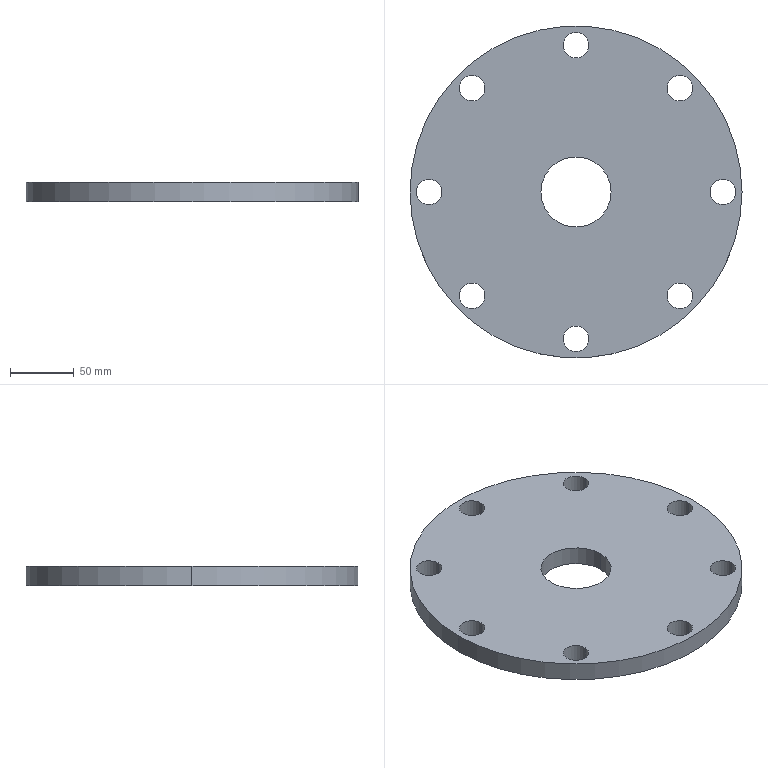Part | SolidWorks | features CirPattern 1, Cut 1, Extrusion 1 | 1 solid | 22 faces | box 260 x 260 x 15 mm | volume 723057 mm3 | cylinder 20 | plane 2 | commonest cylinder face diameters 20 x16 55 x2 260 x2
STEP:
#1=CARTESIAN_POINT('',(-10.,115.,0.));
#2=VERTEX_POINT('',#1);
#3=CARTESIAN_POINT('',(10.,115.,0.));
#4=VERTEX_POINT('',#3);
#5=CARTESIAN_POINT('',(0.,115.,0.));
#6=DIRECTION('',(0.,0.,1.));
#7=DIRECTION('',(1.,0.,0.));
#8=AXIS2_PLACEMENT_3D('',#5,#6,#7);
#9=CIRCLE('',#8,10.);
#10=EDGE_CURVE('',#2,#4,#9,.T.);
#11=ORIENTED_EDGE('',*,*,#10,.F.);
#12=CARTESIAN_POINT('',(-10.,115.,15.));
#13=VERTEX_POINT('',#12);
#14=CARTESIAN_POINT('',(-10.,115.,-0.000012));
#15=DIRECTION('',(0.,0.,1.));
#16=VECTOR('',#15,1000.);
#17=LINE('',#14,#16);
#18=EDGE_CURVE('',#2,#13,#17,.T.);
#19=ORIENTED_EDGE('',*,*,#18,.T.);
#20=CARTESIAN_POINT('',(10.,115.,15.));
#21=VERTEX_POINT('',#20);
#22=CARTESIAN_POINT('',(0.,115.,15.));
#23=DIRECTION('',(0.,0.,1.));
#24=DIRECTION('',(0.,-1.,0.));
#25=AXIS2_PLACEMENT_3D('',#22,#23,#24);
#26=CIRCLE('',#25,10.);
#27=EDGE_CURVE('',#13,#21,#26,.T.);
#28=ORIENTED_EDGE('',*,*,#27,.T.);
#29=CARTESIAN_POINT('',(10.,115.,-0.000012));
#30=DIRECTION('',(0.,0.,1.));
#31=VECTOR('',#30,1000.);
#32=LINE('',#29,#31);
#33=EDGE_CURVE('',#4,#21,#32,.T.);
#34=ORIENTED_EDGE('',*,*,#33,.F.);
#35=EDGE_LOOP('',(#11,#19,#28,#34));
#36=FACE_OUTER_BOUND('',#35,.T.);
#37=CARTESIAN_POINT('',(0.,115.,-0.000012));
#38=DIRECTION('',(0.,0.,1.));
#39=DIRECTION('',(1.,0.,0.));
#40=AXIS2_PLACEMENT_3D('',#37,#38,#39);
#41=CYLINDRICAL_SURFACE('',#40,10.);
#42=ADVANCED_FACE('',(#36),#41,.F.);
#43=CARTESIAN_POINT('',(71.317,81.317,0.));
#44=VERTEX_POINT('',#43);
#45=CARTESIAN_POINT('',(91.317,81.317,0.));
#46=VERTEX_POINT('',#45);
#47=CARTESIAN_POINT('',(81.317,81.317,0.));
#48=DIRECTION('',(0.,0.,1.));
#49=DIRECTION('',(1.,0.,0.));
#50=AXIS2_PLACEMENT_3D('',#47,#48,#49);
#51=CIRCLE('',#50,10.);
#52=EDGE_CURVE('',#44,#46,#51,.T.);
#53=ORIENTED_EDGE('',*,*,#52,.F.);
#54=CARTESIAN_POINT('',(71.317,81.317,15.));
#55=VERTEX_POINT('',#54);
#56=CARTESIAN_POINT('',(71.317,81.317,-0.000012));
#57=DIRECTION('',(0.,0.,1.));
#58=VECTOR('',#57,1000.);
#59=LINE('',#56,#58);
#60=EDGE_CURVE('',#44,#55,#59,.T.);
#61=ORIENTED_EDGE('',*,*,#60,.T.);
#62=CARTESIAN_POINT('',(91.317,81.317,15.));
#63=VERTEX_POINT('',#62);
#64=CARTESIAN_POINT('',(81.317,81.317,15.));
#65=DIRECTION('',(0.,0.,1.));
#66=DIRECTION('',(-0.7071,-0.7071,0.));
#67=AXIS2_PLACEMENT_3D('',#64,#65,#66);
#68=CIRCLE('',#67,10.);
#69=EDGE_CURVE('',#55,#63,#68,.T.);
#70=ORIENTED_EDGE('',*,*,#69,.T.);
#71=CARTESIAN_POINT('',(91.317,81.317,-0.000012));
#72=DIRECTION('',(0.,0.,1.));
#73=VECTOR('',#72,1000.);
#74=LINE('',#71,#73);
#75=EDGE_CURVE('',#46,#63,#74,.T.);
#76=ORIENTED_EDGE('',*,*,#75,.F.);
#77=EDGE_LOOP('',(#53,#61,#70,#76));
#78=FACE_OUTER_BOUND('',#77,.T.);
#79=CARTESIAN_POINT('',(81.317,81.317,-0.000012));
#80=DIRECTION('',(0.,0.,1.));
#81=DIRECTION('',(1.,0.,0.));
#82=AXIS2_PLACEMENT_3D('',#79,#80,#81);
#83=CYLINDRICAL_SURFACE('',#82,10.);
#84=ADVANCED_FACE('',(#78),#83,.F.);
#85=CARTESIAN_POINT('',(105.,0.,0.));
#86=VERTEX_POINT('',#85);
#87=CARTESIAN_POINT('',(125.,0.,0.));
#88=VERTEX_POINT('',#87);
#89=CARTESIAN_POINT('',(115.,0.,0.));
#90=DIRECTION('',(0.,0.,1.));
#91=DIRECTION('',(1.,0.,0.));
#92=AXIS2_PLACEMENT_3D('',#89,#90,#91);
#93=CIRCLE('',#92,10.);
#94=EDGE_CURVE('',#86,#88,#93,.T.);
#95=ORIENTED_EDGE('',*,*,#94,.F.);
#96=CARTESIAN_POINT('',(105.,0.,15.));
#97=VERTEX_POINT('',#96);
#98=CARTESIAN_POINT('',(105.,0.,-0.000012));
#99=DIRECTION('',(0.,0.,1.));
#100=VECTOR('',#99,1000.);
#101=LINE('',#98,#100);
#102=EDGE_CURVE('',#86,#97,#101,.T.);
#103=ORIENTED_EDGE('',*,*,#102,.T.);
#104=CARTESIAN_POINT('',(125.,0.,15.));
#105=VERTEX_POINT('',#104);
#106=CARTESIAN_POINT('',(115.,0.,15.));
#107=DIRECTION('',(0.,0.,1.));
#108=DIRECTION('',(-1.,0.,0.));
#109=AXIS2_PLACEMENT_3D('',#106,#107,#108);
#110=CIRCLE('',#109,10.);
#111=EDGE_CURVE('',#97,#105,#110,.T.);
#112=ORIENTED_EDGE('',*,*,#111,.T.);
#113=CARTESIAN_POINT('',(125.,0.,-0.000012));
#114=DIRECTION('',(0.,0.,1.));
#115=VECTOR('',#114,1000.);
#116=LINE('',#113,#115);
#117=EDGE_CURVE('',#88,#105,#116,.T.);
#118=ORIENTED_EDGE('',*,*,#117,.F.);
#119=EDGE_LOOP('',(#95,#103,#112,#118));
#120=FACE_OUTER_BOUND('',#119,.T.);
#121=CARTESIAN_POINT('',(115.,0.,-0.000012));
#122=DIRECTION('',(0.,0.,1.));
#123=DIRECTION('',(1.,0.,0.));
#124=AXIS2_PLACEMENT_3D('',#121,#122,#123);
#125=CYLINDRICAL_SURFACE('',#124,10.);
#126=ADVANCED_FACE('',(#120),#125,.F.);
#127=CARTESIAN_POINT('',(71.317,-81.317,0.));
#128=VERTEX_POINT('',#127);
#129=CARTESIAN_POINT('',(91.317,-81.317,0.));
#130=VERTEX_POINT('',#129);
#131=CARTESIAN_POINT('',(81.317,-81.317,0.));
#132=DIRECTION('',(0.,0.,1.));
#133=DIRECTION('',(1.,0.,0.));
#134=AXIS2_PLACEMENT_3D('',#131,#132,#133);
#135=CIRCLE('',#134,10.);
#136=EDGE_CURVE('',#128,#130,#135,.T.);
#137=ORIENTED_EDGE('',*,*,#136,.F.);
#138=CARTESIAN_POINT('',(71.317,-81.317,15.));
#139=VERTEX_POINT('',#138);
#140=CARTESIAN_POINT('',(71.317,-81.317,-0.000012));
#141=DIRECTION('',(0.,0.,1.));
#142=VECTOR('',#141,1000.);
#143=LINE('',#140,#142);
#144=EDGE_CURVE('',#128,#139,#143,.T.);
#145=ORIENTED_EDGE('',*,*,#144,.T.);
#146=CARTESIAN_POINT('',(91.317,-81.317,15.));
#147=VERTEX_POINT('',#146);
#148=CARTESIAN_POINT('',(81.317,-81.317,15.));
#149=DIRECTION('',(0.,0.,1.));
#150=DIRECTION('',(-0.7071,0.7071,0.));
#151=AXIS2_PLACEMENT_3D('',#148,#149,#150);
#152=CIRCLE('',#151,10.);
#153=EDGE_CURVE('',#139,#147,#152,.T.);
#154=ORIENTED_EDGE('',*,*,#153,.T.);
#155=CARTESIAN_POINT('',(91.317,-81.317,-0.000012));
#156=DIRECTION('',(0.,0.,1.));
#157=VECTOR('',#156,1000.);
#158=LINE('',#155,#157);
#159=EDGE_CURVE('',#130,#147,#158,.T.);
#160=ORIENTED_EDGE('',*,*,#159,.F.);
#161=EDGE_LOOP('',(#137,#145,#154,#160));
#162=FACE_OUTER_BOUND('',#161,.T.);
#163=CARTESIAN_POINT('',(81.317,-81.317,-0.000012));
#164=DIRECTION('',(0.,0.,1.));
#165=DIRECTION('',(1.,0.,0.));
#166=AXIS2_PLACEMENT_3D('',#163,#164,#165);
#167=CYLINDRICAL_SURFACE('',#166,10.);
#168=ADVANCED_FACE('',(#162),#167,.F.);
#169=CARTESIAN_POINT('',(-10.,-115.,0.));
#170=VERTEX_POINT('',#169);
#171=CARTESIAN_POINT('',(10.,-115.,0.));
#172=VERTEX_POINT('',#171);
#173=CARTESIAN_POINT('',(0.,-115.,0.));
#174=DIRECTION('',(0.,0.,1.));
#175=DIRECTION('',(1.,0.,0.));
#176=AXIS2_PLACEMENT_3D('',#173,#174,#175);
#177=CIRCLE('',#176,10.);
#178=EDGE_CURVE('',#170,#172,#177,.T.);
#179=ORIENTED_EDGE('',*,*,#178,.F.);
#180=CARTESIAN_POINT('',(-10.,-115.,15.));
#181=VERTEX_POINT('',#180);
#182=CARTESIAN_POINT('',(-10.,-115.,-0.000012));
#183=DIRECTION('',(0.,0.,1.));
#184=VECTOR('',#183,1000.);
#185=LINE('',#182,#184);
#186=EDGE_CURVE('',#170,#181,#185,.T.);
#187=ORIENTED_EDGE('',*,*,#186,.T.);
#188=CARTESIAN_POINT('',(10.,-115.,15.));
#189=VERTEX_POINT('',#188);
#190=CARTESIAN_POINT('',(0.,-115.,15.));
#191=DIRECTION('',(0.,0.,1.));
#192=DIRECTION('',(0.,1.,0.));
#193=AXIS2_PLACEMENT_3D('',#190,#191,#192);
#194=CIRCLE('',#193,10.);
#195=EDGE_CURVE('',#181,#189,#194,.T.);
#196=ORIENTED_EDGE('',*,*,#195,.T.);
#197=CARTESIAN_POINT('',(10.,-115.,-0.000012));
#198=DIRECTION('',(0.,0.,1.));
#199=VECTOR('',#198,1000.);
#200=LINE('',#197,#199);
#201=EDGE_CURVE('',#172,#189,#200,.T.);
#202=ORIENTED_EDGE('',*,*,#201,.F.);
#203=EDGE_LOOP('',(#179,#187,#196,#202));
#204=FACE_OUTER_BOUND('',#203,.T.);
#205=CARTESIAN_POINT('',(0.,-115.,-0.000012));
#206=DIRECTION('',(0.,0.,1.));
#207=DIRECTION('',(1.,0.,0.));
#208=AXIS2_PLACEMENT_3D('',#205,#206,#207);
#209=CYLINDRICAL_SURFACE('',#208,10.);
#210=ADVANCED_FACE('',(#204),#209,.F.);
#211=CARTESIAN_POINT('',(-91.317,-81.317,0.));
#212=VERTEX_POINT('',#211);
#213=CARTESIAN_POINT('',(-71.317,-81.317,0.));
#214=VERTEX_POINT('',#213);
#215=CARTESIAN_POINT('',(-81.317,-81.317,0.));
#216=DIRECTION('',(0.,0.,1.));
#217=DIRECTION('',(1.,0.,0.));
#218=AXIS2_PLACEMENT_3D('',#215,#216,#217);
#219=CIRCLE('',#218,10.);
#220=EDGE_CURVE('',#212,#214,#219,.T.);
#221=ORIENTED_EDGE('',*,*,#220,.F.);
#222=CARTESIAN_POINT('',(-91.317,-81.317,15.));
#223=VERTEX_POINT('',#222);
#224=CARTESIAN_POINT('',(-91.317,-81.317,-0.000012));
#225=DIRECTION('',(0.,0.,1.));
#226=VECTOR('',#225,1000.);
#227=LINE('',#224,#226);
#228=EDGE_CURVE('',#212,#223,#227,.T.);
#229=ORIENTED_EDGE('',*,*,#228,.T.);
#230=CARTESIAN_POINT('',(-71.317,-81.317,15.));
#231=VERTEX_POINT('',#230);
#232=CARTESIAN_POINT('',(-81.317,-81.317,15.));
#233=DIRECTION('',(0.,0.,1.));
#234=DIRECTION('',(0.7071,0.7071,0.));
#235=AXIS2_PLACEMENT_3D('',#232,#233,#234);
#236=CIRCLE('',#235,10.);
#237=EDGE_CURVE('',#223,#231,#236,.T.);
#238=ORIENTED_EDGE('',*,*,#237,.T.);
#239=CARTESIAN_POINT('',(-71.317,-81.317,-0.000012));
#240=DIRECTION('',(0.,0.,1.));
#241=VECTOR('',#240,1000.);
#242=LINE('',#239,#241);
#243=EDGE_CURVE('',#214,#231,#242,.T.);
#244=ORIENTED_EDGE('',*,*,#243,.F.);
#245=EDGE_LOOP('',(#221,#229,#238,#244));
#246=FACE_OUTER_BOUND('',#245,.T.);
#247=CARTESIAN_POINT('',(-81.317,-81.317,-0.000012));
#248=DIRECTION('',(0.,0.,1.));
#249=DIRECTION('',(1.,0.,0.));
#250=AXIS2_PLACEMENT_3D('',#247,#248,#249);
#251=CYLINDRICAL_SURFACE('',#250,10.);
#252=ADVANCED_FACE('',(#246),#251,.F.);
#253=CARTESIAN_POINT('',(-91.317,81.317,0.));
#254=VERTEX_POINT('',#253);
#255=CARTESIAN_POINT('',(-71.317,81.317,0.));
#256=VERTEX_POINT('',#255);
#257=CARTESIAN_POINT('',(-81.317,81.317,0.));
#258=DIRECTION('',(0.,0.,1.));
#259=DIRECTION('',(1.,0.,0.));
#260=AXIS2_PLACEMENT_3D('',#257,#258,#259);
#261=CIRCLE('',#260,10.);
#262=EDGE_CURVE('',#254,#256,#261,.T.);
#263=ORIENTED_EDGE('',*,*,#262,.F.);
#264=CARTESIAN_POINT('',(-91.317,81.317,15.));
#265=VERTEX_POINT('',#264);
#266=CARTESIAN_POINT('',(-91.317,81.317,-0.000012));
#267=DIRECTION('',(0.,0.,1.));
#268=VECTOR('',#267,1000.);
#269=LINE('',#266,#268);
#270=EDGE_CURVE('',#254,#265,#269,.T.);
#271=ORIENTED_EDGE('',*,*,#270,.T.);
#272=CARTESIAN_POINT('',(-71.317,81.317,15.));
#273=VERTEX_POINT('',#272);
#274=CARTESIAN_POINT('',(-81.317,81.317,15.));
#275=DIRECTION('',(0.,0.,1.));
#276=DIRECTION('',(0.7071,-0.7071,0.));
#277=AXIS2_PLACEMENT_3D('',#274,#275,#276);
#278=CIRCLE('',#277,10.);
#279=EDGE_CURVE('',#265,#273,#278,.T.);
#280=ORIENTED_EDGE('',*,*,#279,.T.);
#281=CARTESIAN_POINT('',(-71.317,81.317,-0.000012));
#282=DIRECTION('',(0.,0.,1.));
#283=VECTOR('',#282,1000.);
#284=LINE('',#281,#283);
#285=EDGE_CURVE('',#256,#273,#284,.T.);
#286=ORIENTED_EDGE('',*,*,#285,.F.);
#287=EDGE_LOOP('',(#263,#271,#280,#286));
#288=FACE_OUTER_BOUND('',#287,.T.);
#289=CARTESIAN_POINT('',(-81.317,81.317,-0.000012));
#290=DIRECTION('',(0.,0.,1.));
#291=DIRECTION('',(1.,0.,0.));
#292=AXIS2_PLACEMENT_3D('',#289,#290,#291);
#293=CYLINDRICAL_SURFACE('',#292,10.);
#294=ADVANCED_FACE('',(#288),#293,.F.);
#295=CARTESIAN_POINT('',(-125.,0.,0.));
#296=VERTEX_POINT('',#295);
#297=CARTESIAN_POINT('',(-105.,0.,0.));
#298=VERTEX_POINT('',#297);
#299=CARTESIAN_POINT('',(-115.,0.,0.));
#300=DIRECTION('',(0.,0.,1.));
#301=DIRECTION('',(1.,0.,0.));
#302=AXIS2_PLACEMENT_3D('',#299,#300,#301);
#303=CIRCLE('',#302,10.);
#304=EDGE_CURVE('',#296,#298,#303,.T.);
#305=ORIENTED_EDGE('',*,*,#304,.F.);
#306=CARTESIAN_POINT('',(-125.,0.,15.));
#307=VERTEX_POINT('',#306);
#308=CARTESIAN_POINT('',(-125.,0.,-0.000012));
#309=DIRECTION('',(0.,0.,1.));
#310=VECTOR('',#309,1000.);
#311=LINE('',#308,#310);
#312=EDGE_CURVE('',#296,#307,#311,.T.);
#313=ORIENTED_EDGE('',*,*,#312,.T.);
#314=CARTESIAN_POINT('',(-105.,0.,15.));
#315=VERTEX_POINT('',#314);
#316=CARTESIAN_POINT('',(-115.,0.,15.));
#317=DIRECTION('',(0.,0.,1.));
#318=DIRECTION('',(1.,0.,0.));
#319=AXIS2_PLACEMENT_3D('',#316,#317,#318);
#320=CIRCLE('',#319,10.);
#321=EDGE_CURVE('',#307,#315,#320,.T.);
#322=ORIENTED_EDGE('',*,*,#321,.T.);
#323=CARTESIAN_POINT('',(-105.,0.,-0.000012));
#324=DIRECTION('',(0.,0.,1.));
#325=VECTOR('',#324,1000.);
#326=LINE('',#323,#325);
#327=EDGE_CURVE('',#298,#315,#326,.T.);
#328=ORIENTED_EDGE('',*,*,#327,.F.);
#329=EDGE_LOOP('',(#305,#313,#322,#328));
#330=FACE_OUTER_BOUND('',#329,.T.);
#331=CARTESIAN_POINT('',(-115.,0.,-0.000012));
#332=DIRECTION('',(0.,0.,1.));
#333=DIRECTION('',(1.,0.,0.));
#334=AXIS2_PLACEMENT_3D('',#331,#332,#333);
#335=CYLINDRICAL_SURFACE('',#334,10.);
#336=ADVANCED_FACE('',(#330),#335,.F.);
#337=CARTESIAN_POINT('',(-27.5,0.,15.));
#338=VERTEX_POINT('',#337);
#339=CARTESIAN_POINT('',(27.5,0.,15.));
#340=VERTEX_POINT('',#339);
#341=CARTESIAN_POINT('',(0.,0.,15.));
#342=DIRECTION('',(0.,0.,1.));
#343=DIRECTION('',(1.,0.,0.));
#344=AXIS2_PLACEMENT_3D('',#341,#342,#343);
#345=CIRCLE('',#344,27.5);
#346=EDGE_CURVE('',#338,#340,#345,.T.);
#347=ORIENTED_EDGE('',*,*,#346,.T.);
#348=CARTESIAN_POINT('',(27.5,0.,0.));
#349=VERTEX_POINT('',#348);
#350=CARTESIAN_POINT('',(27.5,0.,15.));
#351=DIRECTION('',(0.,0.,-1.));
#352=VECTOR('',#351,1000.);
#353=LINE('',#350,#352);
#354=EDGE_CURVE('',#340,#349,#353,.T.);
#355=ORIENTED_EDGE('',*,*,#354,.T.);
#356=CARTESIAN_POINT('',(-27.5,0.,0.));
#357=VERTEX_POINT('',#356);
#358=CARTESIAN_POINT('',(0.,0.,0.));
#359=DIRECTION('',(0.,0.,1.));
#360=DIRECTION('',(1.,0.,0.));
#361=AXIS2_PLACEMENT_3D('',#358,#359,#360);
#362=CIRCLE('',#361,27.5);
#363=EDGE_CURVE('',#357,#349,#362,.T.);
#364=ORIENTED_EDGE('',*,*,#363,.F.);
#365=CARTESIAN_POINT('',(-27.5,0.,15.));
#366=DIRECTION('',(0.,0.,-1.));
#367=VECTOR('',#366,1000.);
#368=LINE('',#365,#367);
#369=EDGE_CURVE('',#338,#357,#368,.T.);
#370=ORIENTED_EDGE('',*,*,#369,.F.);
#371=EDGE_LOOP('',(#347,#355,#364,#370));
#372=FACE_OUTER_BOUND('',#371,.T.);
#373=CARTESIAN_POINT('',(0.,0.,15.));
#374=DIRECTION('',(0.,0.,-1.));
#375=DIRECTION('',(-1.,0.,0.));
#376=AXIS2_PLACEMENT_3D('',#373,#374,#375);
#377=CYLINDRICAL_SURFACE('',#376,27.5);
#378=ADVANCED_FACE('',(#372),#377,.F.);
#379=CARTESIAN_POINT('',(130.,0.,15.));
#380=VERTEX_POINT('',#379);
#381=CARTESIAN_POINT('',(-130.,0.,15.));
#382=VERTEX_POINT('',#381);
#383=CARTESIAN_POINT('',(0.,0.,15.));
#384=DIRECTION('',(0.,0.,1.));
#385=DIRECTION('',(1.,0.,0.));
#386=AXIS2_PLACEMENT_3D('',#383,#384,#385);
#387=CIRCLE('',#386,130.);
#388=EDGE_CURVE('',#380,#382,#387,.T.);
#389=ORIENTED_EDGE('',*,*,#388,.F.);
#390=CARTESIAN_POINT('',(130.,0.,0.));
#391=VERTEX_POINT('',#390);
#392=CARTESIAN_POINT('',(130.,0.,15.));
#393=DIRECTION('',(0.,0.,-1.));
#394=VECTOR('',#393,1000.);
#395=LINE('',#392,#394);
#396=EDGE_CURVE('',#380,#391,#395,.T.);
#397=ORIENTED_EDGE('',*,*,#396,.T.);
#398=CARTESIAN_POINT('',(-130.,0.,0.));
#399=VERTEX_POINT('',#398);
#400=CARTESIAN_POINT('',(0.,0.,0.));
#401=DIRECTION('',(0.,0.,1.));
#402=DIRECTION('',(1.,0.,0.));
#403=AXIS2_PLACEMENT_3D('',#400,#401,#402);
#404=CIRCLE('',#403,130.);
#405=EDGE_CURVE('',#391,#399,#404,.T.);
#406=ORIENTED_EDGE('',*,*,#405,.T.);
#407=CARTESIAN_POINT('',(-130.,0.,15.));
#408=DIRECTION('',(0.,0.,-1.));
#409=VECTOR('',#408,1000.);
#410=LINE('',#407,#409);
#411=EDGE_CURVE('',#382,#399,#410,.T.);
#412=ORIENTED_EDGE('',*,*,#411,.F.);
#413=EDGE_LOOP('',(#389,#397,#406,#412));
#414=FACE_OUTER_BOUND('',#413,.T.);
#415=CARTESIAN_POINT('',(0.,0.,15.));
#416=DIRECTION('',(0.,0.,-1.));
#417=DIRECTION('',(-1.,0.,0.));
#418=AXIS2_PLACEMENT_3D('',#415,#416,#417);
#419=CYLINDRICAL_SURFACE('',#418,130.);
#420=ADVANCED_FACE('',(#414),#419,.T.);
#421=CARTESIAN_POINT('',(0.,115.,15.));
#422=DIRECTION('',(0.,0.,1.));
#423=DIRECTION('',(0.,-1.,0.));
#424=AXIS2_PLACEMENT_3D('',#421,#422,#423);
#425=CIRCLE('',#424,10.);
#426=EDGE_CURVE('',#21,#13,#425,.T.);
#427=ORIENTED_EDGE('',*,*,#426,.F.);
#428=ORIENTED_EDGE('',*,*,#27,.F.);
#429=EDGE_LOOP('',(#427,#428));
#430=FACE_BOUND('',#429,.T.);
#431=CARTESIAN_POINT('',(81.317,81.317,15.));
#432=DIRECTION('',(0.,0.,1.));
#433=DIRECTION('',(-0.7071,-0.7071,0.));
#434=AXIS2_PLACEMENT_3D('',#431,#432,#433);
#435=CIRCLE('',#434,10.);
#436=EDGE_CURVE('',#63,#55,#435,.T.);
#437=ORIENTED_EDGE('',*,*,#436,.F.);
#438=ORIENTED_EDGE('',*,*,#69,.F.);
#439=EDGE_LOOP('',(#437,#438));
#440=FACE_BOUND('',#439,.T.);
#441=CARTESIAN_POINT('',(115.,0.,15.));
#442=DIRECTION('',(0.,0.,1.));
#443=DIRECTION('',(-1.,0.,0.));
#444=AXIS2_PLACEMENT_3D('',#441,#442,#443);
#445=CIRCLE('',#444,10.);
#446=EDGE_CURVE('',#105,#97,#445,.T.);
#447=ORIENTED_EDGE('',*,*,#446,.F.);
#448=ORIENTED_EDGE('',*,*,#111,.F.);
#449=EDGE_LOOP('',(#447,#448));
#450=FACE_BOUND('',#449,.T.);
#451=CARTESIAN_POINT('',(81.317,-81.317,15.));
#452=DIRECTION('',(0.,0.,1.));
#453=DIRECTION('',(-0.7071,0.7071,0.));
#454=AXIS2_PLACEMENT_3D('',#451,#452,#453);
#455=CIRCLE('',#454,10.);
#456=EDGE_CURVE('',#147,#139,#455,.T.);
#457=ORIENTED_EDGE('',*,*,#456,.F.);
#458=ORIENTED_EDGE('',*,*,#153,.F.);
#459=EDGE_LOOP('',(#457,#458));
#460=FACE_BOUND('',#459,.T.);
#461=CARTESIAN_POINT('',(0.,-115.,15.));
#462=DIRECTION('',(0.,0.,1.));
#463=DIRECTION('',(0.,1.,0.));
#464=AXIS2_PLACEMENT_3D('',#461,#462,#463);
#465=CIRCLE('',#464,10.);
#466=EDGE_CURVE('',#189,#181,#465,.T.);
#467=ORIENTED_EDGE('',*,*,#466,.F.);
#468=ORIENTED_EDGE('',*,*,#195,.F.);
#469=EDGE_LOOP('',(#467,#468));
#470=FACE_BOUND('',#469,.T.);
#471=CARTESIAN_POINT('',(-81.317,-81.317,15.));
#472=DIRECTION('',(0.,0.,1.));
#473=DIRECTION('',(0.7071,0.7071,0.));
#474=AXIS2_PLACEMENT_3D('',#471,#472,#473);
#475=CIRCLE('',#474,10.);
#476=EDGE_CURVE('',#231,#223,#475,.T.);
#477=ORIENTED_EDGE('',*,*,#476,.F.);
#478=ORIENTED_EDGE('',*,*,#237,.F.);
#479=EDGE_LOOP('',(#477,#478));
#480=FACE_BOUND('',#479,.T.);
#481=CARTESIAN_POINT('',(-81.317,81.317,15.));
#482=DIRECTION('',(0.,0.,1.));
#483=DIRECTION('',(0.7071,-0.7071,0.));
#484=AXIS2_PLACEMENT_3D('',#481,#482,#483);
#485=CIRCLE('',#484,10.);
#486=EDGE_CURVE('',#273,#265,#485,.T.);
#487=ORIENTED_EDGE('',*,*,#486,.F.);
#488=ORIENTED_EDGE('',*,*,#279,.F.);
#489=EDGE_LOOP('',(#487,#488));
#490=FACE_BOUND('',#489,.T.);
#491=CARTESIAN_POINT('',(-115.,0.,15.));
#492=DIRECTION('',(0.,0.,1.));
#493=DIRECTION('',(1.,0.,0.));
#494=AXIS2_PLACEMENT_3D('',#491,#492,#493);
#495=CIRCLE('',#494,10.);
#496=EDGE_CURVE('',#315,#307,#495,.T.);
#497=ORIENTED_EDGE('',*,*,#496,.F.);
#498=ORIENTED_EDGE('',*,*,#321,.F.);
#499=EDGE_LOOP('',(#497,#498));
#500=FACE_BOUND('',#499,.T.);
#501=CARTESIAN_POINT('',(0.,0.,15.));
#502=DIRECTION('',(0.,0.,1.));
#503=DIRECTION('',(1.,0.,0.));
#504=AXIS2_PLACEMENT_3D('',#501,#502,#503);
#505=CIRCLE('',#504,130.);
#506=EDGE_CURVE('',#382,#380,#505,.T.);
#507=ORIENTED_EDGE('',*,*,#506,.T.);
#508=ORIENTED_EDGE('',*,*,#388,.T.);
#509=EDGE_LOOP('',(#507,#508));
#510=FACE_OUTER_BOUND('',#509,.T.);
#511=ORIENTED_EDGE('',*,*,#346,.F.);
#512=CARTESIAN_POINT('',(0.,0.,15.));
#513=DIRECTION('',(0.,0.,1.));
#514=DIRECTION('',(1.,0.,0.));
#515=AXIS2_PLACEMENT_3D('',#512,#513,#514);
#516=CIRCLE('',#515,27.5);
#517=EDGE_CURVE('',#340,#338,#516,.T.);
#518=ORIENTED_EDGE('',*,*,#517,.F.);
#519=EDGE_LOOP('',(#511,#518));
#520=FACE_BOUND('',#519,.T.);
#521=CARTESIAN_POINT('',(0.,0.,15.));
#522=DIRECTION('',(0.,0.,1.));
#523=DIRECTION('',(1.,0.,0.));
#524=AXIS2_PLACEMENT_3D('',#521,#522,#523);
#525=PLANE('',#524);
#526=ADVANCED_FACE('',(#430,#440,#450,#460,#470,#480,#490,#500,#510,#520),#525,.T.);
#527=CARTESIAN_POINT('',(0.,115.,0.));
#528=DIRECTION('',(0.,0.,1.));
#529=DIRECTION('',(1.,0.,0.));
#530=AXIS2_PLACEMENT_3D('',#527,#528,#529);
#531=CIRCLE('',#530,10.);
#532=EDGE_CURVE('',#4,#2,#531,.T.);
#533=ORIENTED_EDGE('',*,*,#532,.T.);
#534=ORIENTED_EDGE('',*,*,#10,.T.);
#535=EDGE_LOOP('',(#533,#534));
#536=FACE_BOUND('',#535,.T.);
#537=CARTESIAN_POINT('',(81.317,81.317,0.));
#538=DIRECTION('',(0.,0.,1.));
#539=DIRECTION('',(1.,0.,0.));
#540=AXIS2_PLACEMENT_3D('',#537,#538,#539);
#541=CIRCLE('',#540,10.);
#542=EDGE_CURVE('',#46,#44,#541,.T.);
#543=ORIENTED_EDGE('',*,*,#542,.T.);
#544=ORIENTED_EDGE('',*,*,#52,.T.);
#545=EDGE_LOOP('',(#543,#544));
#546=FACE_BOUND('',#545,.T.);
#547=CARTESIAN_POINT('',(115.,0.,0.));
#548=DIRECTION('',(0.,0.,1.));
#549=DIRECTION('',(1.,0.,0.));
#550=AXIS2_PLACEMENT_3D('',#547,#548,#549);
#551=CIRCLE('',#550,10.);
#552=EDGE_CURVE('',#88,#86,#551,.T.);
#553=ORIENTED_EDGE('',*,*,#552,.T.);
#554=ORIENTED_EDGE('',*,*,#94,.T.);
#555=EDGE_LOOP('',(#553,#554));
#556=FACE_BOUND('',#555,.T.);
#557=CARTESIAN_POINT('',(81.317,-81.317,0.));
#558=DIRECTION('',(0.,0.,1.));
#559=DIRECTION('',(1.,0.,0.));
#560=AXIS2_PLACEMENT_3D('',#557,#558,#559);
#561=CIRCLE('',#560,10.);
#562=EDGE_CURVE('',#130,#128,#561,.T.);
#563=ORIENTED_EDGE('',*,*,#562,.T.);
#564=ORIENTED_EDGE('',*,*,#136,.T.);
#565=EDGE_LOOP('',(#563,#564));
#566=FACE_BOUND('',#565,.T.);
#567=CARTESIAN_POINT('',(0.,-115.,0.));
#568=DIRECTION('',(0.,0.,1.));
#569=DIRECTION('',(1.,0.,0.));
#570=AXIS2_PLACEMENT_3D('',#567,#568,#569);
#571=CIRCLE('',#570,10.);
#572=EDGE_CURVE('',#172,#170,#571,.T.);
#573=ORIENTED_EDGE('',*,*,#572,.T.);
#574=ORIENTED_EDGE('',*,*,#178,.T.);
#575=EDGE_LOOP('',(#573,#574));
#576=FACE_BOUND('',#575,.T.);
#577=CARTESIAN_POINT('',(-81.317,-81.317,0.));
#578=DIRECTION('',(0.,0.,1.));
#579=DIRECTION('',(1.,0.,0.));
#580=AXIS2_PLACEMENT_3D('',#577,#578,#579);
#581=CIRCLE('',#580,10.);
#582=EDGE_CURVE('',#214,#212,#581,.T.);
#583=ORIENTED_EDGE('',*,*,#582,.T.);
#584=ORIENTED_EDGE('',*,*,#220,.T.);
#585=EDGE_LOOP('',(#583,#584));
#586=FACE_BOUND('',#585,.T.);
#587=CARTESIAN_POINT('',(-81.317,81.317,0.));
#588=DIRECTION('',(0.,0.,1.));
#589=DIRECTION('',(1.,0.,0.));
#590=AXIS2_PLACEMENT_3D('',#587,#588,#589);
#591=CIRCLE('',#590,10.);
#592=EDGE_CURVE('',#256,#254,#591,.T.);
#593=ORIENTED_EDGE('',*,*,#592,.T.);
#594=ORIENTED_EDGE('',*,*,#262,.T.);
#595=EDGE_LOOP('',(#593,#594));
#596=FACE_BOUND('',#595,.T.);
#597=CARTESIAN_POINT('',(-115.,0.,0.));
#598=DIRECTION('',(0.,0.,1.));
#599=DIRECTION('',(1.,0.,0.));
#600=AXIS2_PLACEMENT_3D('',#597,#598,#599);
#601=CIRCLE('',#600,10.);
#602=EDGE_CURVE('',#298,#296,#601,.T.);
#603=ORIENTED_EDGE('',*,*,#602,.T.);
#604=ORIENTED_EDGE('',*,*,#304,.T.);
#605=EDGE_LOOP('',(#603,#604));
#606=FACE_BOUND('',#605,.T.);
#607=CARTESIAN_POINT('',(0.,0.,0.));
#608=DIRECTION('',(0.,0.,1.));
#609=DIRECTION('',(1.,0.,0.));
#610=AXIS2_PLACEMENT_3D('',#607,#608,#609);
#611=CIRCLE('',#610,130.);
#612=EDGE_CURVE('',#399,#391,#611,.T.);
#613=ORIENTED_EDGE('',*,*,#612,.F.);
#614=ORIENTED_EDGE('',*,*,#405,.F.);
#615=EDGE_LOOP('',(#613,#614));
#616=FACE_OUTER_BOUND('',#615,.T.);
#617=ORIENTED_EDGE('',*,*,#363,.T.);
#618=CARTESIAN_POINT('',(0.,0.,0.));
#619=DIRECTION('',(0.,0.,1.));
#620=DIRECTION('',(1.,0.,0.));
#621=AXIS2_PLACEMENT_3D('',#618,#619,#620);
#622=CIRCLE('',#621,27.5);
#623=EDGE_CURVE('',#349,#357,#622,.T.);
#624=ORIENTED_EDGE('',*,*,#623,.T.);
#625=EDGE_LOOP('',(#617,#624));
#626=FACE_BOUND('',#625,.T.);
#627=CARTESIAN_POINT('',(0.,0.,0.));
#628=DIRECTION('',(0.,0.,1.));
#629=DIRECTION('',(1.,0.,0.));
#630=AXIS2_PLACEMENT_3D('',#627,#628,#629);
#631=PLANE('',#630);
#632=ADVANCED_FACE('',(#536,#546,#556,#566,#576,#586,#596,#606,#616,#626),#631,.F.);
#633=ORIENTED_EDGE('',*,*,#396,.F.);
#634=ORIENTED_EDGE('',*,*,#506,.F.);
#635=ORIENTED_EDGE('',*,*,#411,.T.);
#636=ORIENTED_EDGE('',*,*,#612,.T.);
#637=EDGE_LOOP('',(#633,#634,#635,#636));
#638=FACE_OUTER_BOUND('',#637,.T.);
#639=CARTESIAN_POINT('',(0.,0.,15.));
#640=DIRECTION('',(0.,0.,-1.));
#641=DIRECTION('',(-1.,0.,0.));
#642=AXIS2_PLACEMENT_3D('',#639,#640,#641);
#643=CYLINDRICAL_SURFACE('',#642,130.);
#644=ADVANCED_FACE('',(#638),#643,.T.);
#645=ORIENTED_EDGE('',*,*,#354,.F.);
#646=ORIENTED_EDGE('',*,*,#517,.T.);
#647=ORIENTED_EDGE('',*,*,#369,.T.);
#648=ORIENTED_EDGE('',*,*,#623,.F.);
#649=EDGE_LOOP('',(#645,#646,#647,#648));
#650=FACE_OUTER_BOUND('',#649,.T.);
#651=CARTESIAN_POINT('',(0.,0.,15.));
#652=DIRECTION('',(0.,0.,-1.));
#653=DIRECTION('',(-1.,0.,0.));
#654=AXIS2_PLACEMENT_3D('',#651,#652,#653);
#655=CYLINDRICAL_SURFACE('',#654,27.5);
#656=ADVANCED_FACE('',(#650),#655,.F.);
#657=ORIENTED_EDGE('',*,*,#312,.F.);
#658=ORIENTED_EDGE('',*,*,#602,.F.);
#659=ORIENTED_EDGE('',*,*,#327,.T.);
#660=ORIENTED_EDGE('',*,*,#496,.T.);
#661=EDGE_LOOP('',(#657,#658,#659,#660));
#662=FACE_OUTER_BOUND('',#661,.T.);
#663=CARTESIAN_POINT('',(-115.,0.,-0.000012));
#664=DIRECTION('',(0.,0.,1.));
#665=DIRECTION('',(1.,0.,0.));
#666=AXIS2_PLACEMENT_3D('',#663,#664,#665);
#667=CYLINDRICAL_SURFACE('',#666,10.);
#668=ADVANCED_FACE('',(#662),#667,.F.);
#669=ORIENTED_EDGE('',*,*,#270,.F.);
#670=ORIENTED_EDGE('',*,*,#592,.F.);
#671=ORIENTED_EDGE('',*,*,#285,.T.);
#672=ORIENTED_EDGE('',*,*,#486,.T.);
#673=EDGE_LOOP('',(#669,#670,#671,#672));
#674=FACE_OUTER_BOUND('',#673,.T.);
#675=CARTESIAN_POINT('',(-81.317,81.317,-0.000012));
#676=DIRECTION('',(0.,0.,1.));
#677=DIRECTION('',(1.,0.,0.));
#678=AXIS2_PLACEMENT_3D('',#675,#676,#677);
#679=CYLINDRICAL_SURFACE('',#678,10.);
#680=ADVANCED_FACE('',(#674),#679,.F.);
#681=ORIENTED_EDGE('',*,*,#228,.F.);
#682=ORIENTED_EDGE('',*,*,#582,.F.);
#683=ORIENTED_EDGE('',*,*,#243,.T.);
#684=ORIENTED_EDGE('',*,*,#476,.T.);
#685=EDGE_LOOP('',(#681,#682,#683,#684));
#686=FACE_OUTER_BOUND('',#685,.T.);
#687=CARTESIAN_POINT('',(-81.317,-81.317,-0.000012));
#688=DIRECTION('',(0.,0.,1.));
#689=DIRECTION('',(1.,0.,0.));
#690=AXIS2_PLACEMENT_3D('',#687,#688,#689);
#691=CYLINDRICAL_SURFACE('',#690,10.);
#692=ADVANCED_FACE('',(#686),#691,.F.);
#693=ORIENTED_EDGE('',*,*,#186,.F.);
#694=ORIENTED_EDGE('',*,*,#572,.F.);
#695=ORIENTED_EDGE('',*,*,#201,.T.);
#696=ORIENTED_EDGE('',*,*,#466,.T.);
#697=EDGE_LOOP('',(#693,#694,#695,#696));
#698=FACE_OUTER_BOUND('',#697,.T.);
#699=CARTESIAN_POINT('',(0.,-115.,-0.000012));
#700=DIRECTION('',(0.,0.,1.));
#701=DIRECTION('',(1.,0.,0.));
#702=AXIS2_PLACEMENT_3D('',#699,#700,#701);
#703=CYLINDRICAL_SURFACE('',#702,10.);
#704=ADVANCED_FACE('',(#698),#703,.F.);
#705=ORIENTED_EDGE('',*,*,#144,.F.);
#706=ORIENTED_EDGE('',*,*,#562,.F.);
#707=ORIENTED_EDGE('',*,*,#159,.T.);
#708=ORIENTED_EDGE('',*,*,#456,.T.);
#709=EDGE_LOOP('',(#705,#706,#707,#708));
#710=FACE_OUTER_BOUND('',#709,.T.);
#711=CARTESIAN_POINT('',(81.317,-81.317,-0.000012));
#712=DIRECTION('',(0.,0.,1.));
#713=DIRECTION('',(1.,0.,0.));
#714=AXIS2_PLACEMENT_3D('',#711,#712,#713);
#715=CYLINDRICAL_SURFACE('',#714,10.);
#716=ADVANCED_FACE('',(#710),#715,.F.);
#717=ORIENTED_EDGE('',*,*,#102,.F.);
#718=ORIENTED_EDGE('',*,*,#552,.F.);
#719=ORIENTED_EDGE('',*,*,#117,.T.);
#720=ORIENTED_EDGE('',*,*,#446,.T.);
#721=EDGE_LOOP('',(#717,#718,#719,#720));
#722=FACE_OUTER_BOUND('',#721,.T.);
#723=CARTESIAN_POINT('',(115.,0.,-0.000012));
#724=DIRECTION('',(0.,0.,1.));
#725=DIRECTION('',(1.,0.,0.));
#726=AXIS2_PLACEMENT_3D('',#723,#724,#725);
#727=CYLINDRICAL_SURFACE('',#726,10.);
#728=ADVANCED_FACE('',(#722),#727,.F.);
#729=ORIENTED_EDGE('',*,*,#60,.F.);
#730=ORIENTED_EDGE('',*,*,#542,.F.);
#731=ORIENTED_EDGE('',*,*,#75,.T.);
#732=ORIENTED_EDGE('',*,*,#436,.T.);
#733=EDGE_LOOP('',(#729,#730,#731,#732));
#734=FACE_OUTER_BOUND('',#733,.T.);
#735=CARTESIAN_POINT('',(81.317,81.317,-0.000012));
#736=DIRECTION('',(0.,0.,1.));
#737=DIRECTION('',(1.,0.,0.));
#738=AXIS2_PLACEMENT_3D('',#735,#736,#737);
#739=CYLINDRICAL_SURFACE('',#738,10.);
#740=ADVANCED_FACE('',(#734),#739,.F.);
#741=ORIENTED_EDGE('',*,*,#18,.F.);
#742=ORIENTED_EDGE('',*,*,#532,.F.);
#743=ORIENTED_EDGE('',*,*,#33,.T.);
#744=ORIENTED_EDGE('',*,*,#426,.T.);
#745=EDGE_LOOP('',(#741,#742,#743,#744));
#746=FACE_OUTER_BOUND('',#745,.T.);
#747=CARTESIAN_POINT('',(0.,115.,-0.000012));
#748=DIRECTION('',(0.,0.,1.));
#749=DIRECTION('',(1.,0.,0.));
#750=AXIS2_PLACEMENT_3D('',#747,#748,#749);
#751=CYLINDRICAL_SURFACE('',#750,10.);
#752=ADVANCED_FACE('',(#746),#751,.F.);
#753=CLOSED_SHELL('',(#42,#84,#126,#168,#210,#252,#294,#336,#378,#420,#526,#632,#644,#656,#668,#680,#692,#704,#716,#728,#740,#752));
#754=MANIFOLD_SOLID_BREP('',#753);
#755=CARTESIAN_POINT('',(0.,0.,0.));
#756=DIRECTION('',(0.,0.,1.));
#757=DIRECTION('',(1.,0.,0.));
#758=AXIS2_PLACEMENT_3D('',#755,#756,#757);
#759=(LENGTH_UNIT()NAMED_UNIT(*)SI_UNIT(.MILLI.,.METRE.));
#760=UNCERTAINTY_MEASURE_WITH_UNIT(LENGTH_MEASURE(0.00001),#759,'','');
#761=(NAMED_UNIT(*)PLANE_ANGLE_UNIT()SI_UNIT($,.RADIAN.));
#762=(NAMED_UNIT(*)SI_UNIT($,.STERADIAN.)SOLID_ANGLE_UNIT());
#763=(GEOMETRIC_REPRESENTATION_CONTEXT(3)GLOBAL_UNCERTAINTY_ASSIGNED_CONTEXT((#760))GLOBAL_UNIT_ASSIGNED_CONTEXT((#759,#761,#762))REPRESENTATION_CONTEXT('',''));
#764=ADVANCED_BREP_SHAPE_REPRESENTATION('',(#754,#758),#763);